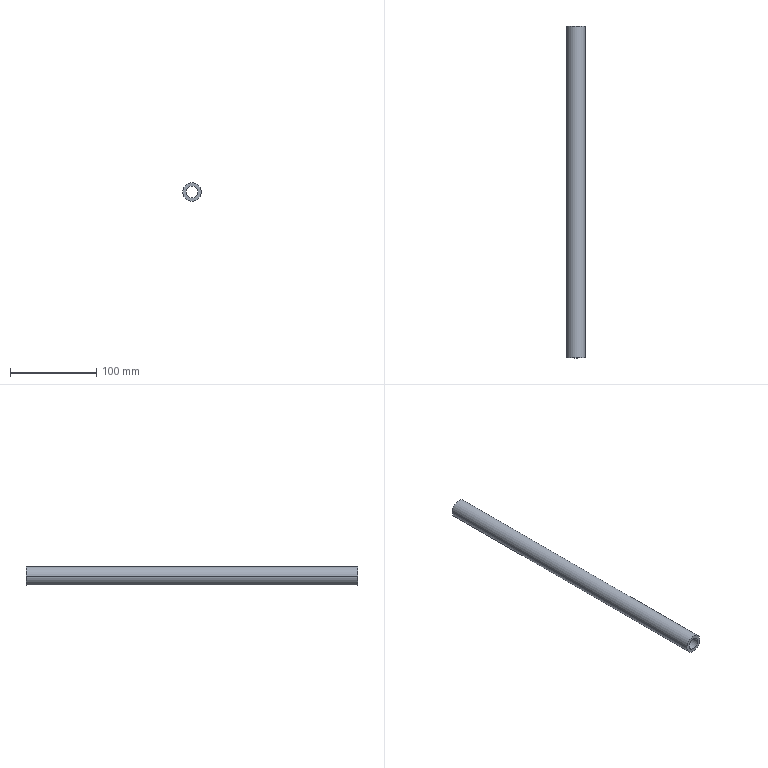Part | SolidWorks | features BaseBody 1 | 1 solid | 6 faces | box 21.234 x 384.6 x 21.234 mm | volume 78104 mm3 | cylinder 4 | plane 2 | commonest cylinder face diameters 13.868 x2 21.234 x2
STEP:
#1=CARTESIAN_POINT('',(-28.118,12.7,0.));
#2=VERTEX_POINT('',#1);
#3=CARTESIAN_POINT('',(-41.986,12.7,0.));
#4=VERTEX_POINT('',#3);
#5=CARTESIAN_POINT('',(-35.052,12.7,0.));
#6=DIRECTION('',(0.,-1.,0.));
#7=DIRECTION('',(1.,0.,0.));
#8=AXIS2_PLACEMENT_3D('',#5,#6,#7);
#9=CIRCLE('',#8,6.934);
#10=EDGE_CURVE('',#2,#4,#9,.T.);
#11=ORIENTED_EDGE('',*,*,#10,.F.);
#12=CARTESIAN_POINT('',(-35.052,12.7,0.));
#13=DIRECTION('',(0.,-1.,0.));
#14=DIRECTION('',(-1.,0.,0.));
#15=AXIS2_PLACEMENT_3D('',#12,#13,#14);
#16=CIRCLE('',#15,6.934);
#17=EDGE_CURVE('',#4,#2,#16,.T.);
#18=ORIENTED_EDGE('',*,*,#17,.F.);
#19=EDGE_LOOP('',(#11,#18));
#20=FACE_BOUND('',#19,.T.);
#21=CARTESIAN_POINT('',(-24.435,12.7,0.));
#22=VERTEX_POINT('',#21);
#23=CARTESIAN_POINT('',(-45.669,12.7,0.));
#24=VERTEX_POINT('',#23);
#25=CARTESIAN_POINT('',(-35.052,12.7,0.));
#26=DIRECTION('',(0.,1.,0.));
#27=DIRECTION('',(1.,0.,0.));
#28=AXIS2_PLACEMENT_3D('',#25,#26,#27);
#29=CIRCLE('',#28,10.617);
#30=EDGE_CURVE('',#22,#24,#29,.T.);
#31=ORIENTED_EDGE('',*,*,#30,.F.);
#32=CARTESIAN_POINT('',(-35.052,12.7,0.));
#33=DIRECTION('',(0.,1.,0.));
#34=DIRECTION('',(-1.,0.,0.));
#35=AXIS2_PLACEMENT_3D('',#32,#33,#34);
#36=CIRCLE('',#35,10.617);
#37=EDGE_CURVE('',#24,#22,#36,.T.);
#38=ORIENTED_EDGE('',*,*,#37,.F.);
#39=EDGE_LOOP('',(#31,#38));
#40=FACE_OUTER_BOUND('',#39,.T.);
#41=CARTESIAN_POINT('',(-35.052,12.7,0.));
#42=DIRECTION('',(0.,-1.,0.));
#43=DIRECTION('',(-1.,0.,0.));
#44=AXIS2_PLACEMENT_3D('',#41,#42,#43);
#45=PLANE('',#44);
#46=ADVANCED_FACE('',(#20,#40),#45,.T.);
#47=CARTESIAN_POINT('',(-28.118,397.3,0.));
#48=VERTEX_POINT('',#47);
#49=CARTESIAN_POINT('',(-41.986,397.3,0.));
#50=VERTEX_POINT('',#49);
#51=CARTESIAN_POINT('',(-35.052,397.3,0.));
#52=DIRECTION('',(0.,1.,0.));
#53=DIRECTION('',(1.,0.,0.));
#54=AXIS2_PLACEMENT_3D('',#51,#52,#53);
#55=CIRCLE('',#54,6.934);
#56=EDGE_CURVE('',#48,#50,#55,.T.);
#57=ORIENTED_EDGE('',*,*,#56,.F.);
#58=CARTESIAN_POINT('',(-35.052,397.3,0.));
#59=DIRECTION('',(0.,1.,0.));
#60=DIRECTION('',(-1.,0.,0.));
#61=AXIS2_PLACEMENT_3D('',#58,#59,#60);
#62=CIRCLE('',#61,6.934);
#63=EDGE_CURVE('',#50,#48,#62,.T.);
#64=ORIENTED_EDGE('',*,*,#63,.F.);
#65=EDGE_LOOP('',(#57,#64));
#66=FACE_BOUND('',#65,.T.);
#67=CARTESIAN_POINT('',(-24.435,397.3,0.));
#68=VERTEX_POINT('',#67);
#69=CARTESIAN_POINT('',(-45.669,397.3,0.));
#70=VERTEX_POINT('',#69);
#71=CARTESIAN_POINT('',(-35.052,397.3,0.));
#72=DIRECTION('',(0.,-1.,0.));
#73=DIRECTION('',(1.,0.,0.));
#74=AXIS2_PLACEMENT_3D('',#71,#72,#73);
#75=CIRCLE('',#74,10.617);
#76=EDGE_CURVE('',#68,#70,#75,.T.);
#77=ORIENTED_EDGE('',*,*,#76,.F.);
#78=CARTESIAN_POINT('',(-35.052,397.3,0.));
#79=DIRECTION('',(0.,-1.,0.));
#80=DIRECTION('',(-1.,0.,0.));
#81=AXIS2_PLACEMENT_3D('',#78,#79,#80);
#82=CIRCLE('',#81,10.617);
#83=EDGE_CURVE('',#70,#68,#82,.T.);
#84=ORIENTED_EDGE('',*,*,#83,.F.);
#85=EDGE_LOOP('',(#77,#84));
#86=FACE_OUTER_BOUND('',#85,.T.);
#87=CARTESIAN_POINT('',(-35.052,397.3,0.));
#88=DIRECTION('',(0.,1.,0.));
#89=DIRECTION('',(1.,0.,0.));
#90=AXIS2_PLACEMENT_3D('',#87,#88,#89);
#91=PLANE('',#90);
#92=ADVANCED_FACE('',(#66,#86),#91,.T.);
#93=ORIENTED_EDGE('',*,*,#37,.T.);
#94=CARTESIAN_POINT('',(-24.435,397.3,0.));
#95=DIRECTION('',(0.,-1.,0.));
#96=VECTOR('',#95,1000.);
#97=LINE('',#94,#96);
#98=EDGE_CURVE('',#68,#22,#97,.T.);
#99=ORIENTED_EDGE('',*,*,#98,.F.);
#100=ORIENTED_EDGE('',*,*,#76,.T.);
#101=CARTESIAN_POINT('',(-45.669,12.7,0.));
#102=DIRECTION('',(0.,1.,0.));
#103=VECTOR('',#102,1000.);
#104=LINE('',#101,#103);
#105=EDGE_CURVE('',#24,#70,#104,.T.);
#106=ORIENTED_EDGE('',*,*,#105,.F.);
#107=EDGE_LOOP('',(#93,#99,#100,#106));
#108=FACE_OUTER_BOUND('',#107,.T.);
#109=CARTESIAN_POINT('',(-35.052,397.3,0.));
#110=DIRECTION('',(0.,-1.,0.));
#111=DIRECTION('',(1.,0.,0.));
#112=AXIS2_PLACEMENT_3D('',#109,#110,#111);
#113=CYLINDRICAL_SURFACE('',#112,10.617);
#114=ADVANCED_FACE('',(#108),#113,.T.);
#115=ORIENTED_EDGE('',*,*,#105,.T.);
#116=ORIENTED_EDGE('',*,*,#83,.T.);
#117=ORIENTED_EDGE('',*,*,#98,.T.);
#118=ORIENTED_EDGE('',*,*,#30,.T.);
#119=EDGE_LOOP('',(#115,#116,#117,#118));
#120=FACE_OUTER_BOUND('',#119,.T.);
#121=CARTESIAN_POINT('',(-35.052,397.3,0.));
#122=DIRECTION('',(0.,-1.,0.));
#123=DIRECTION('',(1.,0.,0.));
#124=AXIS2_PLACEMENT_3D('',#121,#122,#123);
#125=CYLINDRICAL_SURFACE('',#124,10.617);
#126=ADVANCED_FACE('',(#120),#125,.T.);
#127=ORIENTED_EDGE('',*,*,#17,.T.);
#128=CARTESIAN_POINT('',(-28.118,397.3,0.));
#129=DIRECTION('',(0.,-1.,0.));
#130=VECTOR('',#129,1000.);
#131=LINE('',#128,#130);
#132=EDGE_CURVE('',#48,#2,#131,.T.);
#133=ORIENTED_EDGE('',*,*,#132,.F.);
#134=ORIENTED_EDGE('',*,*,#56,.T.);
#135=CARTESIAN_POINT('',(-41.986,12.7,0.));
#136=DIRECTION('',(0.,1.,0.));
#137=VECTOR('',#136,1000.);
#138=LINE('',#135,#137);
#139=EDGE_CURVE('',#4,#50,#138,.T.);
#140=ORIENTED_EDGE('',*,*,#139,.F.);
#141=EDGE_LOOP('',(#127,#133,#134,#140));
#142=FACE_OUTER_BOUND('',#141,.T.);
#143=CARTESIAN_POINT('',(-35.052,397.3,0.));
#144=DIRECTION('',(0.,-1.,0.));
#145=DIRECTION('',(1.,0.,0.));
#146=AXIS2_PLACEMENT_3D('',#143,#144,#145);
#147=CYLINDRICAL_SURFACE('',#146,6.934);
#148=ADVANCED_FACE('',(#142),#147,.F.);
#149=ORIENTED_EDGE('',*,*,#139,.T.);
#150=ORIENTED_EDGE('',*,*,#63,.T.);
#151=ORIENTED_EDGE('',*,*,#132,.T.);
#152=ORIENTED_EDGE('',*,*,#10,.T.);
#153=EDGE_LOOP('',(#149,#150,#151,#152));
#154=FACE_OUTER_BOUND('',#153,.T.);
#155=CARTESIAN_POINT('',(-35.052,397.3,0.));
#156=DIRECTION('',(0.,-1.,0.));
#157=DIRECTION('',(1.,0.,0.));
#158=AXIS2_PLACEMENT_3D('',#155,#156,#157);
#159=CYLINDRICAL_SURFACE('',#158,6.934);
#160=ADVANCED_FACE('',(#154),#159,.F.);
#161=CLOSED_SHELL('',(#46,#92,#114,#126,#148,#160));
#162=MANIFOLD_SOLID_BREP('',#161);
#163=CARTESIAN_POINT('',(0.,0.,0.));
#164=DIRECTION('',(0.,0.,1.));
#165=DIRECTION('',(1.,0.,0.));
#166=AXIS2_PLACEMENT_3D('',#163,#164,#165);
#167=(LENGTH_UNIT()NAMED_UNIT(*)SI_UNIT(.MILLI.,.METRE.));
#168=UNCERTAINTY_MEASURE_WITH_UNIT(LENGTH_MEASURE(0.00001),#167,'','');
#169=(NAMED_UNIT(*)PLANE_ANGLE_UNIT()SI_UNIT($,.RADIAN.));
#170=(NAMED_UNIT(*)SI_UNIT($,.STERADIAN.)SOLID_ANGLE_UNIT());
#171=(GEOMETRIC_REPRESENTATION_CONTEXT(3)GLOBAL_UNCERTAINTY_ASSIGNED_CONTEXT((#168))GLOBAL_UNIT_ASSIGNED_CONTEXT((#167,#169,#170))REPRESENTATION_CONTEXT('',''));
#172=ADVANCED_BREP_SHAPE_REPRESENTATION('',(#162,#166),#171);